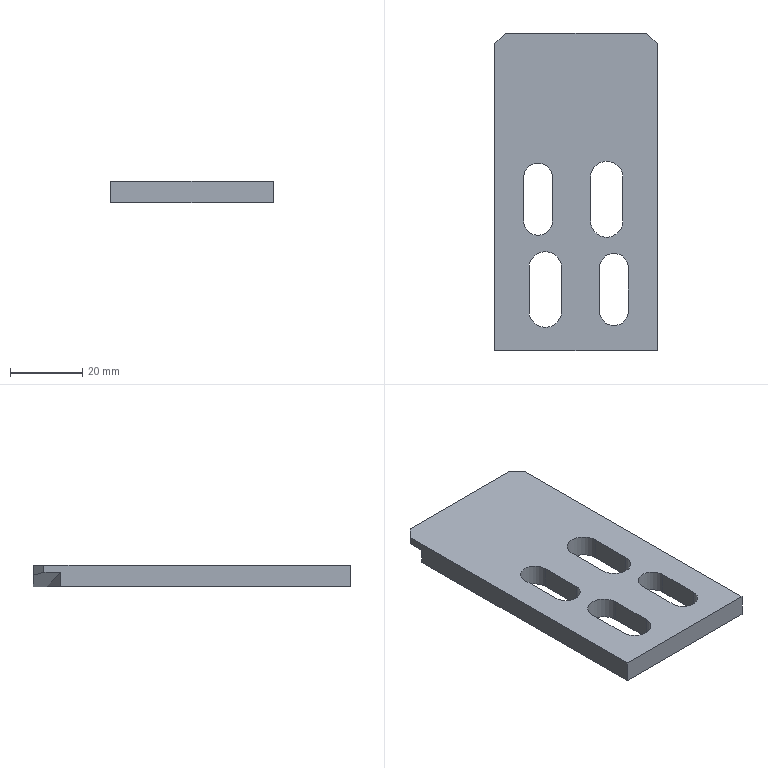Part | STEP file | gslz 2016.10.28-13_id1722_x_t | 1 solid | 28 faces | box 45 x 88 x 6 mm | volume 19661 mm3 | plane 20 | cylinder 8 | commonest cylinder face diameters 8 x4 9 x4